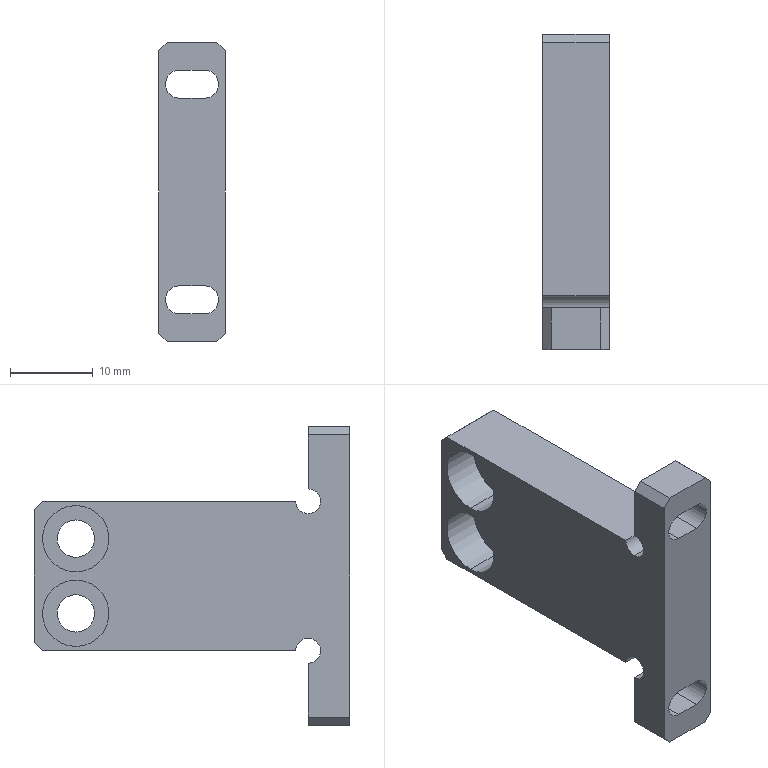Part | SolidWorks | features HoleWzd 2, Chamfer 1, Extrusion 1, ICE 1 | 1 solid | 37 faces | box 8 x 38 x 36 mm | volume 5326 mm3 | plane 22 | cylinder 15 | commonest cylinder face diameters 3.4 x4 4.5 x4 8 x4 3 x3
STEP:
#1=CARTESIAN_POINT('',(4.6,33.,-8.5));
#2=VERTEX_POINT('',#1);
#3=CARTESIAN_POINT('',(4.6,33.,-0.5));
#4=VERTEX_POINT('',#3);
#5=CARTESIAN_POINT('',(4.6,33.,-4.5));
#6=DIRECTION('',(-1.,0.,0.));
#7=DIRECTION('',(0.,0.,1.));
#8=AXIS2_PLACEMENT_3D('',#5,#6,#7);
#9=CIRCLE('',#8,4.);
#10=EDGE_CURVE('',#2,#4,#9,.T.);
#11=ORIENTED_EDGE('',*,*,#10,.F.);
#12=CARTESIAN_POINT('',(0.,33.,-8.5));
#13=VERTEX_POINT('',#12);
#14=CARTESIAN_POINT('',(0.,33.,-8.5));
#15=DIRECTION('',(-1.,0.,0.));
#16=VECTOR('',#15,1000.);
#17=LINE('',#14,#16);
#18=EDGE_CURVE('',#2,#13,#17,.T.);
#19=ORIENTED_EDGE('',*,*,#18,.T.);
#20=CARTESIAN_POINT('',(0.,33.,-0.5));
#21=VERTEX_POINT('',#20);
#22=CARTESIAN_POINT('',(0.,33.,-4.5));
#23=DIRECTION('',(-1.,0.,0.));
#24=DIRECTION('',(0.,0.,1.));
#25=AXIS2_PLACEMENT_3D('',#22,#23,#24);
#26=CIRCLE('',#25,4.);
#27=EDGE_CURVE('',#13,#21,#26,.T.);
#28=ORIENTED_EDGE('',*,*,#27,.T.);
#29=CARTESIAN_POINT('',(0.,33.,-0.5));
#30=DIRECTION('',(-1.,0.,0.));
#31=VECTOR('',#30,1000.);
#32=LINE('',#29,#31);
#33=EDGE_CURVE('',#4,#21,#32,.T.);
#34=ORIENTED_EDGE('',*,*,#33,.F.);
#35=EDGE_LOOP('',(#11,#19,#28,#34));
#36=FACE_OUTER_BOUND('',#35,.T.);
#37=CARTESIAN_POINT('',(0.,33.,-4.5));
#38=DIRECTION('',(-1.,0.,0.));
#39=DIRECTION('',(0.,0.,1.));
#40=AXIS2_PLACEMENT_3D('',#37,#38,#39);
#41=CYLINDRICAL_SURFACE('',#40,4.);
#42=ADVANCED_FACE('',(#36),#41,.F.);
#43=CARTESIAN_POINT('',(8.,33.,-6.75));
#44=VERTEX_POINT('',#43);
#45=CARTESIAN_POINT('',(8.,33.,-2.25));
#46=VERTEX_POINT('',#45);
#47=CARTESIAN_POINT('',(8.,33.,-4.5));
#48=DIRECTION('',(-1.,0.,0.));
#49=DIRECTION('',(0.,0.,1.));
#50=AXIS2_PLACEMENT_3D('',#47,#48,#49);
#51=CIRCLE('',#50,2.25);
#52=EDGE_CURVE('',#44,#46,#51,.T.);
#53=ORIENTED_EDGE('',*,*,#52,.F.);
#54=CARTESIAN_POINT('',(4.6,33.,-6.75));
#55=VERTEX_POINT('',#54);
#56=CARTESIAN_POINT('',(0.,33.,-6.75));
#57=DIRECTION('',(-1.,0.,0.));
#58=VECTOR('',#57,1000.);
#59=LINE('',#56,#58);
#60=EDGE_CURVE('',#44,#55,#59,.T.);
#61=ORIENTED_EDGE('',*,*,#60,.T.);
#62=CARTESIAN_POINT('',(4.6,33.,-2.25));
#63=VERTEX_POINT('',#62);
#64=CARTESIAN_POINT('',(4.6,33.,-4.5));
#65=DIRECTION('',(-1.,0.,0.));
#66=DIRECTION('',(0.,0.,1.));
#67=AXIS2_PLACEMENT_3D('',#64,#65,#66);
#68=CIRCLE('',#67,2.25);
#69=EDGE_CURVE('',#55,#63,#68,.T.);
#70=ORIENTED_EDGE('',*,*,#69,.T.);
#71=CARTESIAN_POINT('',(0.,33.,-2.25));
#72=DIRECTION('',(-1.,0.,0.));
#73=VECTOR('',#72,1000.);
#74=LINE('',#71,#73);
#75=EDGE_CURVE('',#46,#63,#74,.T.);
#76=ORIENTED_EDGE('',*,*,#75,.F.);
#77=EDGE_LOOP('',(#53,#61,#70,#76));
#78=FACE_OUTER_BOUND('',#77,.T.);
#79=CARTESIAN_POINT('',(0.,33.,-4.5));
#80=DIRECTION('',(-1.,0.,0.));
#81=DIRECTION('',(0.,0.,1.));
#82=AXIS2_PLACEMENT_3D('',#79,#80,#81);
#83=CYLINDRICAL_SURFACE('',#82,2.25);
#84=ADVANCED_FACE('',(#78),#83,.F.);
#85=CARTESIAN_POINT('',(4.6,33.,0.5));
#86=VERTEX_POINT('',#85);
#87=CARTESIAN_POINT('',(4.6,33.,8.5));
#88=VERTEX_POINT('',#87);
#89=CARTESIAN_POINT('',(4.6,33.,4.5));
#90=DIRECTION('',(-1.,0.,0.));
#91=DIRECTION('',(0.,0.,1.));
#92=AXIS2_PLACEMENT_3D('',#89,#90,#91);
#93=CIRCLE('',#92,4.);
#94=EDGE_CURVE('',#86,#88,#93,.T.);
#95=ORIENTED_EDGE('',*,*,#94,.F.);
#96=CARTESIAN_POINT('',(0.,33.,0.5));
#97=VERTEX_POINT('',#96);
#98=CARTESIAN_POINT('',(0.,33.,0.5));
#99=DIRECTION('',(-1.,0.,0.));
#100=VECTOR('',#99,1000.);
#101=LINE('',#98,#100);
#102=EDGE_CURVE('',#86,#97,#101,.T.);
#103=ORIENTED_EDGE('',*,*,#102,.T.);
#104=CARTESIAN_POINT('',(0.,33.,8.5));
#105=VERTEX_POINT('',#104);
#106=CARTESIAN_POINT('',(0.,33.,4.5));
#107=DIRECTION('',(-1.,0.,0.));
#108=DIRECTION('',(0.,0.,1.));
#109=AXIS2_PLACEMENT_3D('',#106,#107,#108);
#110=CIRCLE('',#109,4.);
#111=EDGE_CURVE('',#97,#105,#110,.T.);
#112=ORIENTED_EDGE('',*,*,#111,.T.);
#113=CARTESIAN_POINT('',(0.,33.,8.5));
#114=DIRECTION('',(-1.,0.,0.));
#115=VECTOR('',#114,1000.);
#116=LINE('',#113,#115);
#117=EDGE_CURVE('',#88,#105,#116,.T.);
#118=ORIENTED_EDGE('',*,*,#117,.F.);
#119=EDGE_LOOP('',(#95,#103,#112,#118));
#120=FACE_OUTER_BOUND('',#119,.T.);
#121=CARTESIAN_POINT('',(0.,33.,4.5));
#122=DIRECTION('',(-1.,0.,0.));
#123=DIRECTION('',(0.,0.,1.));
#124=AXIS2_PLACEMENT_3D('',#121,#122,#123);
#125=CYLINDRICAL_SURFACE('',#124,4.);
#126=ADVANCED_FACE('',(#120),#125,.F.);
#127=CARTESIAN_POINT('',(8.,33.,2.25));
#128=VERTEX_POINT('',#127);
#129=CARTESIAN_POINT('',(8.,33.,6.75));
#130=VERTEX_POINT('',#129);
#131=CARTESIAN_POINT('',(8.,33.,4.5));
#132=DIRECTION('',(-1.,0.,0.));
#133=DIRECTION('',(0.,0.,1.));
#134=AXIS2_PLACEMENT_3D('',#131,#132,#133);
#135=CIRCLE('',#134,2.25);
#136=EDGE_CURVE('',#128,#130,#135,.T.);
#137=ORIENTED_EDGE('',*,*,#136,.F.);
#138=CARTESIAN_POINT('',(4.6,33.,2.25));
#139=VERTEX_POINT('',#138);
#140=CARTESIAN_POINT('',(0.,33.,2.25));
#141=DIRECTION('',(-1.,0.,0.));
#142=VECTOR('',#141,1000.);
#143=LINE('',#140,#142);
#144=EDGE_CURVE('',#128,#139,#143,.T.);
#145=ORIENTED_EDGE('',*,*,#144,.T.);
#146=CARTESIAN_POINT('',(4.6,33.,6.75));
#147=VERTEX_POINT('',#146);
#148=CARTESIAN_POINT('',(4.6,33.,4.5));
#149=DIRECTION('',(-1.,0.,0.));
#150=DIRECTION('',(0.,0.,1.));
#151=AXIS2_PLACEMENT_3D('',#148,#149,#150);
#152=CIRCLE('',#151,2.25);
#153=EDGE_CURVE('',#139,#147,#152,.T.);
#154=ORIENTED_EDGE('',*,*,#153,.T.);
#155=CARTESIAN_POINT('',(0.,33.,6.75));
#156=DIRECTION('',(-1.,0.,0.));
#157=VECTOR('',#156,1000.);
#158=LINE('',#155,#157);
#159=EDGE_CURVE('',#130,#147,#158,.T.);
#160=ORIENTED_EDGE('',*,*,#159,.F.);
#161=EDGE_LOOP('',(#137,#145,#154,#160));
#162=FACE_OUTER_BOUND('',#161,.T.);
#163=CARTESIAN_POINT('',(0.,33.,4.5));
#164=DIRECTION('',(-1.,0.,0.));
#165=DIRECTION('',(0.,0.,1.));
#166=AXIS2_PLACEMENT_3D('',#163,#164,#165);
#167=CYLINDRICAL_SURFACE('',#166,2.25);
#168=ADVANCED_FACE('',(#162),#167,.F.);
#169=CARTESIAN_POINT('',(0.,5.,7.5));
#170=VERTEX_POINT('',#169);
#171=CARTESIAN_POINT('',(0.,6.5,9.));
#172=VERTEX_POINT('',#171);
#173=CARTESIAN_POINT('',(0.,5.,9.));
#174=DIRECTION('',(1.,0.,0.));
#175=DIRECTION('',(0.,0.,-1.));
#176=AXIS2_PLACEMENT_3D('',#173,#174,#175);
#177=CIRCLE('',#176,1.5);
#178=EDGE_CURVE('',#170,#172,#177,.T.);
#179=ORIENTED_EDGE('',*,*,#178,.F.);
#180=CARTESIAN_POINT('',(8.,5.,7.5));
#181=VERTEX_POINT('',#180);
#182=CARTESIAN_POINT('',(0.,5.,7.5));
#183=DIRECTION('',(1.,0.,0.));
#184=VECTOR('',#183,1000.);
#185=LINE('',#182,#184);
#186=EDGE_CURVE('',#170,#181,#185,.T.);
#187=ORIENTED_EDGE('',*,*,#186,.T.);
#188=CARTESIAN_POINT('',(8.,6.5,9.));
#189=VERTEX_POINT('',#188);
#190=CARTESIAN_POINT('',(8.,5.,9.));
#191=DIRECTION('',(1.,0.,0.));
#192=DIRECTION('',(0.,0.,-1.));
#193=AXIS2_PLACEMENT_3D('',#190,#191,#192);
#194=CIRCLE('',#193,1.5);
#195=EDGE_CURVE('',#181,#189,#194,.T.);
#196=ORIENTED_EDGE('',*,*,#195,.T.);
#197=CARTESIAN_POINT('',(0.,6.5,9.));
#198=DIRECTION('',(1.,0.,0.));
#199=VECTOR('',#198,1000.);
#200=LINE('',#197,#199);
#201=EDGE_CURVE('',#172,#189,#200,.T.);
#202=ORIENTED_EDGE('',*,*,#201,.F.);
#203=EDGE_LOOP('',(#179,#187,#196,#202));
#204=FACE_OUTER_BOUND('',#203,.T.);
#205=CARTESIAN_POINT('',(0.,5.,9.));
#206=DIRECTION('',(1.,0.,0.));
#207=DIRECTION('',(0.,0.,-1.));
#208=AXIS2_PLACEMENT_3D('',#205,#206,#207);
#209=CYLINDRICAL_SURFACE('',#208,1.5);
#210=ADVANCED_FACE('',(#204),#209,.F.);
#211=CARTESIAN_POINT('',(7.,5.,18.));
#212=VERTEX_POINT('',#211);
#213=CARTESIAN_POINT('',(1.,5.,18.));
#214=VERTEX_POINT('',#213);
#215=CARTESIAN_POINT('',(8.,5.,18.));
#216=DIRECTION('',(-1.,0.,0.));
#217=VECTOR('',#216,1000.);
#218=LINE('',#215,#217);
#219=EDGE_CURVE('',#212,#214,#218,.T.);
#220=ORIENTED_EDGE('',*,*,#219,.F.);
#221=CARTESIAN_POINT('',(8.,5.,17.));
#222=VERTEX_POINT('',#221);
#223=CARTESIAN_POINT('',(8.,5.,17.));
#224=DIRECTION('',(0.7071,0.,-0.7071));
#225=VECTOR('',#224,1000.);
#226=LINE('',#223,#225);
#227=EDGE_CURVE('',#212,#222,#226,.T.);
#228=ORIENTED_EDGE('',*,*,#227,.T.);
#229=CARTESIAN_POINT('',(8.,5.,10.5));
#230=VERTEX_POINT('',#229);
#231=CARTESIAN_POINT('',(8.,5.,9.));
#232=DIRECTION('',(0.,0.,1.));
#233=VECTOR('',#232,1000.);
#234=LINE('',#231,#233);
#235=EDGE_CURVE('',#230,#222,#234,.T.);
#236=ORIENTED_EDGE('',*,*,#235,.F.);
#237=CARTESIAN_POINT('',(0.,5.,10.5));
#238=VERTEX_POINT('',#237);
#239=CARTESIAN_POINT('',(0.,5.,10.5));
#240=DIRECTION('',(-1.,0.,0.));
#241=VECTOR('',#240,1000.);
#242=LINE('',#239,#241);
#243=EDGE_CURVE('',#230,#238,#242,.T.);
#244=ORIENTED_EDGE('',*,*,#243,.T.);
#245=CARTESIAN_POINT('',(0.,5.,17.));
#246=VERTEX_POINT('',#245);
#247=CARTESIAN_POINT('',(0.,5.,9.));
#248=DIRECTION('',(0.,0.,1.));
#249=VECTOR('',#248,1000.);
#250=LINE('',#247,#249);
#251=EDGE_CURVE('',#238,#246,#250,.T.);
#252=ORIENTED_EDGE('',*,*,#251,.T.);
#253=CARTESIAN_POINT('',(1.,5.,18.));
#254=DIRECTION('',(0.7071,0.,0.7071));
#255=VECTOR('',#254,1000.);
#256=LINE('',#253,#255);
#257=EDGE_CURVE('',#246,#214,#256,.T.);
#258=ORIENTED_EDGE('',*,*,#257,.T.);
#259=EDGE_LOOP('',(#220,#228,#236,#244,#252,#258));
#260=FACE_OUTER_BOUND('',#259,.T.);
#261=CARTESIAN_POINT('',(2.5,5.,11.3));
#262=VERTEX_POINT('',#261);
#263=CARTESIAN_POINT('',(2.5,5.,14.7));
#264=VERTEX_POINT('',#263);
#265=CARTESIAN_POINT('',(2.5,5.,13.));
#266=DIRECTION('',(0.,1.,0.));
#267=DIRECTION('',(0.,0.,1.));
#268=AXIS2_PLACEMENT_3D('',#265,#266,#267);
#269=CIRCLE('',#268,1.7);
#270=EDGE_CURVE('',#262,#264,#269,.T.);
#271=ORIENTED_EDGE('',*,*,#270,.F.);
#272=CARTESIAN_POINT('',(5.5,5.,11.3));
#273=VERTEX_POINT('',#272);
#274=CARTESIAN_POINT('',(2.5,5.,11.3));
#275=DIRECTION('',(1.,0.,0.));
#276=VECTOR('',#275,1000.);
#277=LINE('',#274,#276);
#278=EDGE_CURVE('',#262,#273,#277,.T.);
#279=ORIENTED_EDGE('',*,*,#278,.T.);
#280=CARTESIAN_POINT('',(5.5,5.,14.7));
#281=VERTEX_POINT('',#280);
#282=CARTESIAN_POINT('',(5.5,5.,13.));
#283=DIRECTION('',(0.,1.,0.));
#284=DIRECTION('',(0.,0.,1.));
#285=AXIS2_PLACEMENT_3D('',#282,#283,#284);
#286=CIRCLE('',#285,1.7);
#287=EDGE_CURVE('',#281,#273,#286,.T.);
#288=ORIENTED_EDGE('',*,*,#287,.F.);
#289=CARTESIAN_POINT('',(2.5,5.,14.7));
#290=DIRECTION('',(1.,0.,0.));
#291=VECTOR('',#290,1000.);
#292=LINE('',#289,#291);
#293=EDGE_CURVE('',#264,#281,#292,.T.);
#294=ORIENTED_EDGE('',*,*,#293,.F.);
#295=EDGE_LOOP('',(#271,#279,#288,#294));
#296=FACE_BOUND('',#295,.T.);
#297=CARTESIAN_POINT('',(8.,5.,9.));
#298=DIRECTION('',(0.,-1.,0.));
#299=DIRECTION('',(0.,0.,-1.));
#300=AXIS2_PLACEMENT_3D('',#297,#298,#299);
#301=PLANE('',#300);
#302=ADVANCED_FACE('',(#260,#296),#301,.F.);
#303=CARTESIAN_POINT('',(0.,6.5,-9.));
#304=VERTEX_POINT('',#303);
#305=CARTESIAN_POINT('',(0.,37.,-9.));
#306=VERTEX_POINT('',#305);
#307=CARTESIAN_POINT('',(0.,38.,-9.));
#308=DIRECTION('',(0.,1.,0.));
#309=VECTOR('',#308,1000.);
#310=LINE('',#307,#309);
#311=EDGE_CURVE('',#304,#306,#310,.T.);
#312=ORIENTED_EDGE('',*,*,#311,.T.);
#313=CARTESIAN_POINT('',(8.,37.,-9.));
#314=VERTEX_POINT('',#313);
#315=CARTESIAN_POINT('',(8.,37.,-9.));
#316=DIRECTION('',(1.,0.,0.));
#317=VECTOR('',#316,1000.);
#318=LINE('',#315,#317);
#319=EDGE_CURVE('',#306,#314,#318,.T.);
#320=ORIENTED_EDGE('',*,*,#319,.T.);
#321=CARTESIAN_POINT('',(8.,6.5,-9.));
#322=VERTEX_POINT('',#321);
#323=CARTESIAN_POINT('',(8.,38.,-9.));
#324=DIRECTION('',(0.,1.,0.));
#325=VECTOR('',#324,1000.);
#326=LINE('',#323,#325);
#327=EDGE_CURVE('',#322,#314,#326,.T.);
#328=ORIENTED_EDGE('',*,*,#327,.F.);
#329=CARTESIAN_POINT('',(0.,6.5,-9.));
#330=DIRECTION('',(-1.,0.,0.));
#331=VECTOR('',#330,1000.);
#332=LINE('',#329,#331);
#333=EDGE_CURVE('',#322,#304,#332,.T.);
#334=ORIENTED_EDGE('',*,*,#333,.T.);
#335=EDGE_LOOP('',(#312,#320,#328,#334));
#336=FACE_OUTER_BOUND('',#335,.T.);
#337=CARTESIAN_POINT('',(8.,38.,-9.));
#338=DIRECTION('',(0.,0.,1.));
#339=DIRECTION('',(0.,-1.,0.));
#340=AXIS2_PLACEMENT_3D('',#337,#338,#339);
#341=PLANE('',#340);
#342=ADVANCED_FACE('',(#336),#341,.F.);
#343=CARTESIAN_POINT('',(0.,38.,-8.));
#344=VERTEX_POINT('',#343);
#345=CARTESIAN_POINT('',(0.,38.,8.));
#346=VERTEX_POINT('',#345);
#347=CARTESIAN_POINT('',(0.,38.,9.));
#348=DIRECTION('',(0.,0.,1.));
#349=VECTOR('',#348,1000.);
#350=LINE('',#347,#349);
#351=EDGE_CURVE('',#344,#346,#350,.T.);
#352=ORIENTED_EDGE('',*,*,#351,.T.);
#353=CARTESIAN_POINT('',(8.,38.,8.));
#354=VERTEX_POINT('',#353);
#355=CARTESIAN_POINT('',(8.,38.,8.));
#356=DIRECTION('',(1.,0.,0.));
#357=VECTOR('',#356,1000.);
#358=LINE('',#355,#357);
#359=EDGE_CURVE('',#346,#354,#358,.T.);
#360=ORIENTED_EDGE('',*,*,#359,.T.);
#361=CARTESIAN_POINT('',(8.,38.,-8.));
#362=VERTEX_POINT('',#361);
#363=CARTESIAN_POINT('',(8.,38.,9.));
#364=DIRECTION('',(0.,0.,1.));
#365=VECTOR('',#364,1000.);
#366=LINE('',#363,#365);
#367=EDGE_CURVE('',#362,#354,#366,.T.);
#368=ORIENTED_EDGE('',*,*,#367,.F.);
#369=CARTESIAN_POINT('',(8.,38.,-8.));
#370=DIRECTION('',(-1.,0.,0.));
#371=VECTOR('',#370,1000.);
#372=LINE('',#369,#371);
#373=EDGE_CURVE('',#362,#344,#372,.T.);
#374=ORIENTED_EDGE('',*,*,#373,.T.);
#375=EDGE_LOOP('',(#352,#360,#368,#374));
#376=FACE_OUTER_BOUND('',#375,.T.);
#377=CARTESIAN_POINT('',(8.,38.,9.));
#378=DIRECTION('',(0.,-1.,0.));
#379=DIRECTION('',(0.,0.,-1.));
#380=AXIS2_PLACEMENT_3D('',#377,#378,#379);
#381=PLANE('',#380);
#382=ADVANCED_FACE('',(#376),#381,.F.);
#383=CARTESIAN_POINT('',(8.,37.,9.));
#384=VERTEX_POINT('',#383);
#385=CARTESIAN_POINT('',(8.,38.,9.));
#386=DIRECTION('',(0.,-1.,0.));
#387=VECTOR('',#386,1000.);
#388=LINE('',#385,#387);
#389=EDGE_CURVE('',#384,#189,#388,.T.);
#390=ORIENTED_EDGE('',*,*,#389,.F.);
#391=CARTESIAN_POINT('',(0.,37.,9.));
#392=VERTEX_POINT('',#391);
#393=CARTESIAN_POINT('',(8.,37.,9.));
#394=DIRECTION('',(-1.,0.,0.));
#395=VECTOR('',#394,1000.);
#396=LINE('',#393,#395);
#397=EDGE_CURVE('',#384,#392,#396,.T.);
#398=ORIENTED_EDGE('',*,*,#397,.T.);
#399=CARTESIAN_POINT('',(0.,38.,9.));
#400=DIRECTION('',(0.,-1.,0.));
#401=VECTOR('',#400,1000.);
#402=LINE('',#399,#401);
#403=EDGE_CURVE('',#392,#172,#402,.T.);
#404=ORIENTED_EDGE('',*,*,#403,.T.);
#405=ORIENTED_EDGE('',*,*,#201,.T.);
#406=EDGE_LOOP('',(#390,#398,#404,#405));
#407=FACE_OUTER_BOUND('',#406,.T.);
#408=CARTESIAN_POINT('',(8.,38.,9.));
#409=DIRECTION('',(0.,0.,-1.));
#410=DIRECTION('',(0.,1.,0.));
#411=AXIS2_PLACEMENT_3D('',#408,#409,#410);
#412=PLANE('',#411);
#413=ADVANCED_FACE('',(#407),#412,.F.);
#414=CARTESIAN_POINT('',(7.,0.,18.));
#415=VERTEX_POINT('',#414);
#416=CARTESIAN_POINT('',(1.,0.,18.));
#417=VERTEX_POINT('',#416);
#418=CARTESIAN_POINT('',(8.,0.,18.));
#419=DIRECTION('',(-1.,0.,0.));
#420=VECTOR('',#419,1000.);
#421=LINE('',#418,#420);
#422=EDGE_CURVE('',#415,#417,#421,.T.);
#423=ORIENTED_EDGE('',*,*,#422,.F.);
#424=CARTESIAN_POINT('',(7.,5.,18.));
#425=DIRECTION('',(0.,1.,0.));
#426=VECTOR('',#425,1000.);
#427=LINE('',#424,#426);
#428=EDGE_CURVE('',#415,#212,#427,.T.);
#429=ORIENTED_EDGE('',*,*,#428,.T.);
#430=ORIENTED_EDGE('',*,*,#219,.T.);
#431=CARTESIAN_POINT('',(1.,5.,18.));
#432=DIRECTION('',(0.,-1.,0.));
#433=VECTOR('',#432,1000.);
#434=LINE('',#431,#433);
#435=EDGE_CURVE('',#214,#417,#434,.T.);
#436=ORIENTED_EDGE('',*,*,#435,.T.);
#437=EDGE_LOOP('',(#423,#429,#430,#436));
#438=FACE_OUTER_BOUND('',#437,.T.);
#439=CARTESIAN_POINT('',(8.,5.,18.));
#440=DIRECTION('',(0.,0.,-1.));
#441=DIRECTION('',(-1.,0.,0.));
#442=AXIS2_PLACEMENT_3D('',#439,#440,#441);
#443=PLANE('',#442);
#444=ADVANCED_FACE('',(#438),#443,.F.);
#445=CARTESIAN_POINT('',(2.5,0.,-11.3));
#446=VERTEX_POINT('',#445);
#447=CARTESIAN_POINT('',(5.5,0.,-11.3));
#448=VERTEX_POINT('',#447);
#449=CARTESIAN_POINT('',(2.5,0.,-11.3));
#450=DIRECTION('',(1.,0.,0.));
#451=VECTOR('',#450,1000.);
#452=LINE('',#449,#451);
#453=EDGE_CURVE('',#446,#448,#452,.T.);
#454=ORIENTED_EDGE('',*,*,#453,.T.);
#455=CARTESIAN_POINT('',(5.5,0.,-14.7));
#456=VERTEX_POINT('',#455);
#457=CARTESIAN_POINT('',(5.5,0.,-13.));
#458=DIRECTION('',(0.,1.,0.));
#459=DIRECTION('',(0.,0.,1.));
#460=AXIS2_PLACEMENT_3D('',#457,#458,#459);
#461=CIRCLE('',#460,1.7);
#462=EDGE_CURVE('',#448,#456,#461,.T.);
#463=ORIENTED_EDGE('',*,*,#462,.T.);
#464=CARTESIAN_POINT('',(2.5,0.,-14.7));
#465=VERTEX_POINT('',#464);
#466=CARTESIAN_POINT('',(2.5,0.,-14.7));
#467=DIRECTION('',(1.,0.,0.));
#468=VECTOR('',#467,1000.);
#469=LINE('',#466,#468);
#470=EDGE_CURVE('',#465,#456,#469,.T.);
#471=ORIENTED_EDGE('',*,*,#470,.F.);
#472=CARTESIAN_POINT('',(2.5,0.,-13.));
#473=DIRECTION('',(0.,1.,0.));
#474=DIRECTION('',(0.,0.,1.));
#475=AXIS2_PLACEMENT_3D('',#472,#473,#474);
#476=CIRCLE('',#475,1.7);
#477=EDGE_CURVE('',#465,#446,#476,.T.);
#478=ORIENTED_EDGE('',*,*,#477,.T.);
#479=EDGE_LOOP('',(#454,#463,#471,#478));
#480=FACE_BOUND('',#479,.T.);
#481=CARTESIAN_POINT('',(2.5,0.,11.3));
#482=VERTEX_POINT('',#481);
#483=CARTESIAN_POINT('',(2.5,0.,14.7));
#484=VERTEX_POINT('',#483);
#485=CARTESIAN_POINT('',(2.5,0.,13.));
#486=DIRECTION('',(0.,1.,0.));
#487=DIRECTION('',(0.,0.,1.));
#488=AXIS2_PLACEMENT_3D('',#485,#486,#487);
#489=CIRCLE('',#488,1.7);
#490=EDGE_CURVE('',#482,#484,#489,.T.);
#491=ORIENTED_EDGE('',*,*,#490,.T.);
#492=CARTESIAN_POINT('',(5.5,0.,14.7));
#493=VERTEX_POINT('',#492);
#494=CARTESIAN_POINT('',(2.5,0.,14.7));
#495=DIRECTION('',(1.,0.,0.));
#496=VECTOR('',#495,1000.);
#497=LINE('',#494,#496);
#498=EDGE_CURVE('',#484,#493,#497,.T.);
#499=ORIENTED_EDGE('',*,*,#498,.T.);
#500=CARTESIAN_POINT('',(5.5,0.,11.3));
#501=VERTEX_POINT('',#500);
#502=CARTESIAN_POINT('',(5.5,0.,13.));
#503=DIRECTION('',(0.,1.,0.));
#504=DIRECTION('',(0.,0.,1.));
#505=AXIS2_PLACEMENT_3D('',#502,#503,#504);
#506=CIRCLE('',#505,1.7);
#507=EDGE_CURVE('',#493,#501,#506,.T.);
#508=ORIENTED_EDGE('',*,*,#507,.T.);
#509=CARTESIAN_POINT('',(2.5,0.,11.3));
#510=DIRECTION('',(1.,0.,0.));
#511=VECTOR('',#510,1000.);
#512=LINE('',#509,#511);
#513=EDGE_CURVE('',#482,#501,#512,.T.);
#514=ORIENTED_EDGE('',*,*,#513,.F.);
#515=EDGE_LOOP('',(#491,#499,#508,#514));
#516=FACE_BOUND('',#515,.T.);
#517=CARTESIAN_POINT('',(7.,0.,-18.));
#518=VERTEX_POINT('',#517);
#519=CARTESIAN_POINT('',(1.,0.,-18.));
#520=VERTEX_POINT('',#519);
#521=CARTESIAN_POINT('',(8.,0.,-18.));
#522=DIRECTION('',(-1.,0.,0.));
#523=VECTOR('',#522,1000.);
#524=LINE('',#521,#523);
#525=EDGE_CURVE('',#518,#520,#524,.T.);
#526=ORIENTED_EDGE('',*,*,#525,.F.);
#527=CARTESIAN_POINT('',(8.,0.,-17.));
#528=VERTEX_POINT('',#527);
#529=CARTESIAN_POINT('',(8.,0.,-17.));
#530=DIRECTION('',(0.7071,0.,0.7071));
#531=VECTOR('',#530,1000.);
#532=LINE('',#529,#531);
#533=EDGE_CURVE('',#518,#528,#532,.T.);
#534=ORIENTED_EDGE('',*,*,#533,.T.);
#535=CARTESIAN_POINT('',(8.,0.,17.));
#536=VERTEX_POINT('',#535);
#537=CARTESIAN_POINT('',(8.,0.,-18.));
#538=DIRECTION('',(0.,0.,-1.));
#539=VECTOR('',#538,1000.);
#540=LINE('',#537,#539);
#541=EDGE_CURVE('',#536,#528,#540,.T.);
#542=ORIENTED_EDGE('',*,*,#541,.F.);
#543=CARTESIAN_POINT('',(8.,0.,17.));
#544=DIRECTION('',(-0.7071,0.,0.7071));
#545=VECTOR('',#544,1000.);
#546=LINE('',#543,#545);
#547=EDGE_CURVE('',#536,#415,#546,.T.);
#548=ORIENTED_EDGE('',*,*,#547,.T.);
#549=ORIENTED_EDGE('',*,*,#422,.T.);
#550=CARTESIAN_POINT('',(0.,0.,17.));
#551=VERTEX_POINT('',#550);
#552=CARTESIAN_POINT('',(1.,0.,18.));
#553=DIRECTION('',(-0.7071,0.,-0.7071));
#554=VECTOR('',#553,1000.);
#555=LINE('',#552,#554);
#556=EDGE_CURVE('',#417,#551,#555,.T.);
#557=ORIENTED_EDGE('',*,*,#556,.T.);
#558=CARTESIAN_POINT('',(0.,0.,-17.));
#559=VERTEX_POINT('',#558);
#560=CARTESIAN_POINT('',(0.,0.,-18.));
#561=DIRECTION('',(0.,0.,-1.));
#562=VECTOR('',#561,1000.);
#563=LINE('',#560,#562);
#564=EDGE_CURVE('',#551,#559,#563,.T.);
#565=ORIENTED_EDGE('',*,*,#564,.T.);
#566=CARTESIAN_POINT('',(1.,0.,-18.));
#567=DIRECTION('',(0.7071,0.,-0.7071));
#568=VECTOR('',#567,1000.);
#569=LINE('',#566,#568);
#570=EDGE_CURVE('',#559,#520,#569,.T.);
#571=ORIENTED_EDGE('',*,*,#570,.T.);
#572=EDGE_LOOP('',(#526,#534,#542,#548,#549,#557,#565,#571));
#573=FACE_OUTER_BOUND('',#572,.T.);
#574=CARTESIAN_POINT('',(8.,0.,-18.));
#575=DIRECTION('',(0.,1.,0.));
#576=DIRECTION('',(0.,0.,1.));
#577=AXIS2_PLACEMENT_3D('',#574,#575,#576);
#578=PLANE('',#577);
#579=ADVANCED_FACE('',(#480,#516,#573),#578,.F.);
#580=CARTESIAN_POINT('',(7.,5.,-18.));
#581=VERTEX_POINT('',#580);
#582=CARTESIAN_POINT('',(1.,5.,-18.));
#583=VERTEX_POINT('',#582);
#584=CARTESIAN_POINT('',(8.,5.,-18.));
#585=DIRECTION('',(-1.,0.,0.));
#586=VECTOR('',#585,1000.);
#587=LINE('',#584,#586);
#588=EDGE_CURVE('',#581,#583,#587,.T.);
#589=ORIENTED_EDGE('',*,*,#588,.F.);
#590=CARTESIAN_POINT('',(7.,0.,-18.));
#591=DIRECTION('',(0.,-1.,0.));
#592=VECTOR('',#591,1000.);
#593=LINE('',#590,#592);
#594=EDGE_CURVE('',#581,#518,#593,.T.);
#595=ORIENTED_EDGE('',*,*,#594,.T.);
#596=ORIENTED_EDGE('',*,*,#525,.T.);
#597=CARTESIAN_POINT('',(1.,5.,-18.));
#598=DIRECTION('',(0.,1.,0.));
#599=VECTOR('',#598,1000.);
#600=LINE('',#597,#599);
#601=EDGE_CURVE('',#520,#583,#600,.T.);
#602=ORIENTED_EDGE('',*,*,#601,.T.);
#603=EDGE_LOOP('',(#589,#595,#596,#602));
#604=FACE_OUTER_BOUND('',#603,.T.);
#605=CARTESIAN_POINT('',(8.,5.,-18.));
#606=DIRECTION('',(0.,0.,1.));
#607=DIRECTION('',(1.,0.,0.));
#608=AXIS2_PLACEMENT_3D('',#605,#606,#607);
#609=PLANE('',#608);
#610=ADVANCED_FACE('',(#604),#609,.F.);
#611=CARTESIAN_POINT('',(2.5,5.,-14.7));
#612=VERTEX_POINT('',#611);
#613=CARTESIAN_POINT('',(2.5,5.,-11.3));
#614=VERTEX_POINT('',#613);
#615=CARTESIAN_POINT('',(2.5,5.,-13.));
#616=DIRECTION('',(0.,1.,0.));
#617=DIRECTION('',(0.,0.,1.));
#618=AXIS2_PLACEMENT_3D('',#615,#616,#617);
#619=CIRCLE('',#618,1.7);
#620=EDGE_CURVE('',#612,#614,#619,.T.);
#621=ORIENTED_EDGE('',*,*,#620,.F.);
#622=CARTESIAN_POINT('',(5.5,5.,-14.7));
#623=VERTEX_POINT('',#622);
#624=CARTESIAN_POINT('',(2.5,5.,-14.7));
#625=DIRECTION('',(1.,0.,0.));
#626=VECTOR('',#625,1000.);
#627=LINE('',#624,#626);
#628=EDGE_CURVE('',#612,#623,#627,.T.);
#629=ORIENTED_EDGE('',*,*,#628,.T.);
#630=CARTESIAN_POINT('',(5.5,5.,-11.3));
#631=VERTEX_POINT('',#630);
#632=CARTESIAN_POINT('',(5.5,5.,-13.));
#633=DIRECTION('',(0.,1.,0.));
#634=DIRECTION('',(0.,0.,1.));
#635=AXIS2_PLACEMENT_3D('',#632,#633,#634);
#636=CIRCLE('',#635,1.7);
#637=EDGE_CURVE('',#631,#623,#636,.T.);
#638=ORIENTED_EDGE('',*,*,#637,.F.);
#639=CARTESIAN_POINT('',(2.5,5.,-11.3));
#640=DIRECTION('',(1.,0.,0.));
#641=VECTOR('',#640,1000.);
#642=LINE('',#639,#641);
#643=EDGE_CURVE('',#614,#631,#642,.T.);
#644=ORIENTED_EDGE('',*,*,#643,.F.);
#645=EDGE_LOOP('',(#621,#629,#638,#644));
#646=FACE_BOUND('',#645,.T.);
#647=CARTESIAN_POINT('',(8.,5.,-17.));
#648=VERTEX_POINT('',#647);
#649=CARTESIAN_POINT('',(8.,5.,-10.5));
#650=VERTEX_POINT('',#649);
#651=CARTESIAN_POINT('',(8.,5.,-9.));
#652=DIRECTION('',(0.,0.,1.));
#653=VECTOR('',#652,1000.);
#654=LINE('',#651,#653);
#655=EDGE_CURVE('',#648,#650,#654,.T.);
#656=ORIENTED_EDGE('',*,*,#655,.F.);
#657=CARTESIAN_POINT('',(8.,5.,-17.));
#658=DIRECTION('',(-0.7071,0.,-0.7071));
#659=VECTOR('',#658,1000.);
#660=LINE('',#657,#659);
#661=EDGE_CURVE('',#648,#581,#660,.T.);
#662=ORIENTED_EDGE('',*,*,#661,.T.);
#663=ORIENTED_EDGE('',*,*,#588,.T.);
#664=CARTESIAN_POINT('',(0.,5.,-17.));
#665=VERTEX_POINT('',#664);
#666=CARTESIAN_POINT('',(1.,5.,-18.));
#667=DIRECTION('',(-0.7071,0.,0.7071));
#668=VECTOR('',#667,1000.);
#669=LINE('',#666,#668);
#670=EDGE_CURVE('',#583,#665,#669,.T.);
#671=ORIENTED_EDGE('',*,*,#670,.T.);
#672=CARTESIAN_POINT('',(0.,5.,-10.5));
#673=VERTEX_POINT('',#672);
#674=CARTESIAN_POINT('',(0.,5.,-9.));
#675=DIRECTION('',(0.,0.,1.));
#676=VECTOR('',#675,1000.);
#677=LINE('',#674,#676);
#678=EDGE_CURVE('',#665,#673,#677,.T.);
#679=ORIENTED_EDGE('',*,*,#678,.T.);
#680=CARTESIAN_POINT('',(0.,5.,-10.5));
#681=DIRECTION('',(1.,0.,0.));
#682=VECTOR('',#681,1000.);
#683=LINE('',#680,#682);
#684=EDGE_CURVE('',#673,#650,#683,.T.);
#685=ORIENTED_EDGE('',*,*,#684,.T.);
#686=EDGE_LOOP('',(#656,#662,#663,#671,#679,#685));
#687=FACE_OUTER_BOUND('',#686,.T.);
#688=CARTESIAN_POINT('',(8.,5.,-9.));
#689=DIRECTION('',(0.,-1.,0.));
#690=DIRECTION('',(0.,0.,-1.));
#691=AXIS2_PLACEMENT_3D('',#688,#689,#690);
#692=PLANE('',#691);
#693=ADVANCED_FACE('',(#646,#687),#692,.F.);
#694=CARTESIAN_POINT('',(8.,33.,-4.5));
#695=DIRECTION('',(-1.,0.,0.));
#696=DIRECTION('',(0.,0.,1.));
#697=AXIS2_PLACEMENT_3D('',#694,#695,#696);
#698=CIRCLE('',#697,2.25);
#699=EDGE_CURVE('',#46,#44,#698,.T.);
#700=ORIENTED_EDGE('',*,*,#699,.T.);
#701=ORIENTED_EDGE('',*,*,#52,.T.);
#702=EDGE_LOOP('',(#700,#701));
#703=FACE_BOUND('',#702,.T.);
#704=CARTESIAN_POINT('',(8.,33.,4.5));
#705=DIRECTION('',(-1.,0.,0.));
#706=DIRECTION('',(0.,0.,1.));
#707=AXIS2_PLACEMENT_3D('',#704,#705,#706);
#708=CIRCLE('',#707,2.25);
#709=EDGE_CURVE('',#130,#128,#708,.T.);
#710=ORIENTED_EDGE('',*,*,#709,.T.);
#711=ORIENTED_EDGE('',*,*,#136,.T.);
#712=EDGE_LOOP('',(#710,#711));
#713=FACE_BOUND('',#712,.T.);
#714=ORIENTED_EDGE('',*,*,#541,.T.);
#715=CARTESIAN_POINT('',(8.,5.,-17.));
#716=DIRECTION('',(0.,1.,0.));
#717=VECTOR('',#716,1000.);
#718=LINE('',#715,#717);
#719=EDGE_CURVE('',#528,#648,#718,.T.);
#720=ORIENTED_EDGE('',*,*,#719,.T.);
#721=ORIENTED_EDGE('',*,*,#655,.T.);
#722=CARTESIAN_POINT('',(8.,5.,-9.));
#723=DIRECTION('',(1.,0.,0.));
#724=DIRECTION('',(0.,0.,1.));
#725=AXIS2_PLACEMENT_3D('',#722,#723,#724);
#726=CIRCLE('',#725,1.5);
#727=EDGE_CURVE('',#322,#650,#726,.T.);
#728=ORIENTED_EDGE('',*,*,#727,.F.);
#729=ORIENTED_EDGE('',*,*,#327,.T.);
#730=CARTESIAN_POINT('',(8.,23.,-23.));
#731=DIRECTION('',(0.,0.7071,0.7071));
#732=VECTOR('',#731,1000.);
#733=LINE('',#730,#732);
#734=EDGE_CURVE('',#314,#362,#733,.T.);
#735=ORIENTED_EDGE('',*,*,#734,.T.);
#736=ORIENTED_EDGE('',*,*,#367,.T.);
#737=CARTESIAN_POINT('',(8.,23.,23.));
#738=DIRECTION('',(0.,-0.7071,0.7071));
#739=VECTOR('',#738,1000.);
#740=LINE('',#737,#739);
#741=EDGE_CURVE('',#354,#384,#740,.T.);
#742=ORIENTED_EDGE('',*,*,#741,.T.);
#743=ORIENTED_EDGE('',*,*,#389,.T.);
#744=ORIENTED_EDGE('',*,*,#195,.F.);
#745=CARTESIAN_POINT('',(8.,5.,9.));
#746=DIRECTION('',(1.,0.,0.));
#747=DIRECTION('',(0.,0.,-1.));
#748=AXIS2_PLACEMENT_3D('',#745,#746,#747);
#749=CIRCLE('',#748,1.5);
#750=EDGE_CURVE('',#230,#181,#749,.T.);
#751=ORIENTED_EDGE('',*,*,#750,.F.);
#752=ORIENTED_EDGE('',*,*,#235,.T.);
#753=CARTESIAN_POINT('',(8.,0.,17.));
#754=DIRECTION('',(0.,-1.,0.));
#755=VECTOR('',#754,1000.);
#756=LINE('',#753,#755);
#757=EDGE_CURVE('',#222,#536,#756,.T.);
#758=ORIENTED_EDGE('',*,*,#757,.T.);
#759=EDGE_LOOP('',(#714,#720,#721,#728,#729,#735,#736,#742,#743,#744,#751,#752,#758));
#760=FACE_OUTER_BOUND('',#759,.T.);
#761=CARTESIAN_POINT('',(8.,0.,0.));
#762=DIRECTION('',(1.,0.,0.));
#763=DIRECTION('',(0.,0.,-1.));
#764=AXIS2_PLACEMENT_3D('',#761,#762,#763);
#765=PLANE('',#764);
#766=ADVANCED_FACE('',(#703,#713,#760),#765,.T.);
#767=CARTESIAN_POINT('',(0.,33.,-4.5));
#768=DIRECTION('',(-1.,0.,0.));
#769=DIRECTION('',(0.,0.,1.));
#770=AXIS2_PLACEMENT_3D('',#767,#768,#769);
#771=CIRCLE('',#770,4.);
#772=EDGE_CURVE('',#21,#13,#771,.T.);
#773=ORIENTED_EDGE('',*,*,#772,.F.);
#774=ORIENTED_EDGE('',*,*,#27,.F.);
#775=EDGE_LOOP('',(#773,#774));
#776=FACE_BOUND('',#775,.T.);
#777=CARTESIAN_POINT('',(0.,33.,4.5));
#778=DIRECTION('',(-1.,0.,0.));
#779=DIRECTION('',(0.,0.,1.));
#780=AXIS2_PLACEMENT_3D('',#777,#778,#779);
#781=CIRCLE('',#780,4.);
#782=EDGE_CURVE('',#105,#97,#781,.T.);
#783=ORIENTED_EDGE('',*,*,#782,.F.);
#784=ORIENTED_EDGE('',*,*,#111,.F.);
#785=EDGE_LOOP('',(#783,#784));
#786=FACE_BOUND('',#785,.T.);
#787=ORIENTED_EDGE('',*,*,#678,.F.);
#788=CARTESIAN_POINT('',(0.,0.,-17.));
#789=DIRECTION('',(0.,-1.,0.));
#790=VECTOR('',#789,1000.);
#791=LINE('',#788,#790);
#792=EDGE_CURVE('',#665,#559,#791,.T.);
#793=ORIENTED_EDGE('',*,*,#792,.T.);
#794=ORIENTED_EDGE('',*,*,#564,.F.);
#795=CARTESIAN_POINT('',(0.,0.,17.));
#796=DIRECTION('',(0.,1.,0.));
#797=VECTOR('',#796,1000.);
#798=LINE('',#795,#797);
#799=EDGE_CURVE('',#551,#246,#798,.T.);
#800=ORIENTED_EDGE('',*,*,#799,.T.);
#801=ORIENTED_EDGE('',*,*,#251,.F.);
#802=CARTESIAN_POINT('',(0.,5.,9.));
#803=DIRECTION('',(1.,0.,0.));
#804=DIRECTION('',(0.,0.,-1.));
#805=AXIS2_PLACEMENT_3D('',#802,#803,#804);
#806=CIRCLE('',#805,1.5);
#807=EDGE_CURVE('',#238,#170,#806,.T.);
#808=ORIENTED_EDGE('',*,*,#807,.T.);
#809=ORIENTED_EDGE('',*,*,#178,.T.);
#810=ORIENTED_EDGE('',*,*,#403,.F.);
#811=CARTESIAN_POINT('',(0.,37.,9.));
#812=DIRECTION('',(0.,0.7071,-0.7071));
#813=VECTOR('',#812,1000.);
#814=LINE('',#811,#813);
#815=EDGE_CURVE('',#392,#346,#814,.T.);
#816=ORIENTED_EDGE('',*,*,#815,.T.);
#817=ORIENTED_EDGE('',*,*,#351,.F.);
#818=CARTESIAN_POINT('',(0.,38.,-8.));
#819=DIRECTION('',(0.,-0.7071,-0.7071));
#820=VECTOR('',#819,1000.);
#821=LINE('',#818,#820);
#822=EDGE_CURVE('',#344,#306,#821,.T.);
#823=ORIENTED_EDGE('',*,*,#822,.T.);
#824=ORIENTED_EDGE('',*,*,#311,.F.);
#825=CARTESIAN_POINT('',(0.,5.,-9.));
#826=DIRECTION('',(1.,0.,0.));
#827=DIRECTION('',(0.,0.,-1.));
#828=AXIS2_PLACEMENT_3D('',#825,#826,#827);
#829=CIRCLE('',#828,1.5);
#830=EDGE_CURVE('',#304,#673,#829,.T.);
#831=ORIENTED_EDGE('',*,*,#830,.T.);
#832=EDGE_LOOP('',(#787,#793,#794,#800,#801,#808,#809,#810,#816,#817,#823,#824,#831));
#833=FACE_OUTER_BOUND('',#832,.T.);
#834=CARTESIAN_POINT('',(0.,0.,0.));
#835=DIRECTION('',(1.,0.,0.));
#836=DIRECTION('',(0.,0.,-1.));
#837=AXIS2_PLACEMENT_3D('',#834,#835,#836);
#838=PLANE('',#837);
#839=ADVANCED_FACE('',(#776,#786,#833),#838,.F.);
#840=ORIENTED_EDGE('',*,*,#727,.T.);
#841=ORIENTED_EDGE('',*,*,#684,.F.);
#842=ORIENTED_EDGE('',*,*,#830,.F.);
#843=ORIENTED_EDGE('',*,*,#333,.F.);
#844=EDGE_LOOP('',(#840,#841,#842,#843));
#845=FACE_OUTER_BOUND('',#844,.T.);
#846=CARTESIAN_POINT('',(0.,5.,-9.));
#847=DIRECTION('',(1.,0.,0.));
#848=DIRECTION('',(0.,0.,-1.));
#849=AXIS2_PLACEMENT_3D('',#846,#847,#848);
#850=CYLINDRICAL_SURFACE('',#849,1.5);
#851=ADVANCED_FACE('',(#845),#850,.F.);
#852=ORIENTED_EDGE('',*,*,#186,.F.);
#853=ORIENTED_EDGE('',*,*,#807,.F.);
#854=ORIENTED_EDGE('',*,*,#243,.F.);
#855=ORIENTED_EDGE('',*,*,#750,.T.);
#856=EDGE_LOOP('',(#852,#853,#854,#855));
#857=FACE_OUTER_BOUND('',#856,.T.);
#858=CARTESIAN_POINT('',(0.,5.,9.));
#859=DIRECTION('',(1.,0.,0.));
#860=DIRECTION('',(0.,0.,-1.));
#861=AXIS2_PLACEMENT_3D('',#858,#859,#860);
#862=CYLINDRICAL_SURFACE('',#861,1.5);
#863=ADVANCED_FACE('',(#857),#862,.F.);
#864=ORIENTED_EDGE('',*,*,#144,.F.);
#865=ORIENTED_EDGE('',*,*,#709,.F.);
#866=ORIENTED_EDGE('',*,*,#159,.T.);
#867=CARTESIAN_POINT('',(4.6,33.,4.5));
#868=DIRECTION('',(-1.,0.,0.));
#869=DIRECTION('',(0.,0.,1.));
#870=AXIS2_PLACEMENT_3D('',#867,#868,#869);
#871=CIRCLE('',#870,2.25);
#872=EDGE_CURVE('',#147,#139,#871,.T.);
#873=ORIENTED_EDGE('',*,*,#872,.T.);
#874=EDGE_LOOP('',(#864,#865,#866,#873));
#875=FACE_OUTER_BOUND('',#874,.T.);
#876=CARTESIAN_POINT('',(0.,33.,4.5));
#877=DIRECTION('',(-1.,0.,0.));
#878=DIRECTION('',(0.,0.,1.));
#879=AXIS2_PLACEMENT_3D('',#876,#877,#878);
#880=CYLINDRICAL_SURFACE('',#879,2.25);
#881=ADVANCED_FACE('',(#875),#880,.F.);
#882=ORIENTED_EDGE('',*,*,#872,.F.);
#883=ORIENTED_EDGE('',*,*,#153,.F.);
#884=EDGE_LOOP('',(#882,#883));
#885=FACE_BOUND('',#884,.T.);
#886=CARTESIAN_POINT('',(4.6,33.,4.5));
#887=DIRECTION('',(-1.,0.,0.));
#888=DIRECTION('',(0.,0.,1.));
#889=AXIS2_PLACEMENT_3D('',#886,#887,#888);
#890=CIRCLE('',#889,4.);
#891=EDGE_CURVE('',#88,#86,#890,.T.);
#892=ORIENTED_EDGE('',*,*,#891,.T.);
#893=ORIENTED_EDGE('',*,*,#94,.T.);
#894=EDGE_LOOP('',(#892,#893));
#895=FACE_OUTER_BOUND('',#894,.T.);
#896=CARTESIAN_POINT('',(4.6,35.25,4.5));
#897=DIRECTION('',(1.,0.,0.));
#898=DIRECTION('',(0.,0.,-1.));
#899=AXIS2_PLACEMENT_3D('',#896,#897,#898);
#900=PLANE('',#899);
#901=ADVANCED_FACE('',(#885,#895),#900,.F.);
#902=ORIENTED_EDGE('',*,*,#102,.F.);
#903=ORIENTED_EDGE('',*,*,#891,.F.);
#904=ORIENTED_EDGE('',*,*,#117,.T.);
#905=ORIENTED_EDGE('',*,*,#782,.T.);
#906=EDGE_LOOP('',(#902,#903,#904,#905));
#907=FACE_OUTER_BOUND('',#906,.T.);
#908=CARTESIAN_POINT('',(0.,33.,4.5));
#909=DIRECTION('',(-1.,0.,0.));
#910=DIRECTION('',(0.,0.,1.));
#911=AXIS2_PLACEMENT_3D('',#908,#909,#910);
#912=CYLINDRICAL_SURFACE('',#911,4.);
#913=ADVANCED_FACE('',(#907),#912,.F.);
#914=ORIENTED_EDGE('',*,*,#60,.F.);
#915=ORIENTED_EDGE('',*,*,#699,.F.);
#916=ORIENTED_EDGE('',*,*,#75,.T.);
#917=CARTESIAN_POINT('',(4.6,33.,-4.5));
#918=DIRECTION('',(-1.,0.,0.));
#919=DIRECTION('',(0.,0.,1.));
#920=AXIS2_PLACEMENT_3D('',#917,#918,#919);
#921=CIRCLE('',#920,2.25);
#922=EDGE_CURVE('',#63,#55,#921,.T.);
#923=ORIENTED_EDGE('',*,*,#922,.T.);
#924=EDGE_LOOP('',(#914,#915,#916,#923));
#925=FACE_OUTER_BOUND('',#924,.T.);
#926=CARTESIAN_POINT('',(0.,33.,-4.5));
#927=DIRECTION('',(-1.,0.,0.));
#928=DIRECTION('',(0.,0.,1.));
#929=AXIS2_PLACEMENT_3D('',#926,#927,#928);
#930=CYLINDRICAL_SURFACE('',#929,2.25);
#931=ADVANCED_FACE('',(#925),#930,.F.);
#932=ORIENTED_EDGE('',*,*,#922,.F.);
#933=ORIENTED_EDGE('',*,*,#69,.F.);
#934=EDGE_LOOP('',(#932,#933));
#935=FACE_BOUND('',#934,.T.);
#936=CARTESIAN_POINT('',(4.6,33.,-4.5));
#937=DIRECTION('',(-1.,0.,0.));
#938=DIRECTION('',(0.,0.,1.));
#939=AXIS2_PLACEMENT_3D('',#936,#937,#938);
#940=CIRCLE('',#939,4.);
#941=EDGE_CURVE('',#4,#2,#940,.T.);
#942=ORIENTED_EDGE('',*,*,#941,.T.);
#943=ORIENTED_EDGE('',*,*,#10,.T.);
#944=EDGE_LOOP('',(#942,#943));
#945=FACE_OUTER_BOUND('',#944,.T.);
#946=CARTESIAN_POINT('',(4.6,35.25,-4.5));
#947=DIRECTION('',(1.,0.,0.));
#948=DIRECTION('',(0.,0.,-1.));
#949=AXIS2_PLACEMENT_3D('',#946,#947,#948);
#950=PLANE('',#949);
#951=ADVANCED_FACE('',(#935,#945),#950,.F.);
#952=ORIENTED_EDGE('',*,*,#18,.F.);
#953=ORIENTED_EDGE('',*,*,#941,.F.);
#954=ORIENTED_EDGE('',*,*,#33,.T.);
#955=ORIENTED_EDGE('',*,*,#772,.T.);
#956=EDGE_LOOP('',(#952,#953,#954,#955));
#957=FACE_OUTER_BOUND('',#956,.T.);
#958=CARTESIAN_POINT('',(0.,33.,-4.5));
#959=DIRECTION('',(-1.,0.,0.));
#960=DIRECTION('',(0.,0.,1.));
#961=AXIS2_PLACEMENT_3D('',#958,#959,#960);
#962=CYLINDRICAL_SURFACE('',#961,4.);
#963=ADVANCED_FACE('',(#957),#962,.F.);
#964=ORIENTED_EDGE('',*,*,#507,.F.);
#965=CARTESIAN_POINT('',(5.5,5.,14.7));
#966=DIRECTION('',(0.,-1.,0.));
#967=VECTOR('',#966,1000.);
#968=LINE('',#965,#967);
#969=EDGE_CURVE('',#281,#493,#968,.T.);
#970=ORIENTED_EDGE('',*,*,#969,.F.);
#971=ORIENTED_EDGE('',*,*,#287,.T.);
#972=CARTESIAN_POINT('',(5.5,5.,11.3));
#973=DIRECTION('',(0.,1.,0.));
#974=VECTOR('',#973,1000.);
#975=LINE('',#972,#974);
#976=EDGE_CURVE('',#501,#273,#975,.T.);
#977=ORIENTED_EDGE('',*,*,#976,.F.);
#978=EDGE_LOOP('',(#964,#970,#971,#977));
#979=FACE_OUTER_BOUND('',#978,.T.);
#980=CARTESIAN_POINT('',(5.5,5.,13.));
#981=DIRECTION('',(0.,1.,0.));
#982=DIRECTION('',(0.,0.,1.));
#983=AXIS2_PLACEMENT_3D('',#980,#981,#982);
#984=CYLINDRICAL_SURFACE('',#983,1.7);
#985=ADVANCED_FACE('',(#979),#984,.F.);
#986=ORIENTED_EDGE('',*,*,#270,.T.);
#987=CARTESIAN_POINT('',(2.5,5.,14.7));
#988=DIRECTION('',(0.,1.,0.));
#989=VECTOR('',#988,1000.);
#990=LINE('',#987,#989);
#991=EDGE_CURVE('',#484,#264,#990,.T.);
#992=ORIENTED_EDGE('',*,*,#991,.F.);
#993=ORIENTED_EDGE('',*,*,#490,.F.);
#994=CARTESIAN_POINT('',(2.5,5.,11.3));
#995=DIRECTION('',(0.,-1.,0.));
#996=VECTOR('',#995,1000.);
#997=LINE('',#994,#996);
#998=EDGE_CURVE('',#262,#482,#997,.T.);
#999=ORIENTED_EDGE('',*,*,#998,.F.);
#1000=EDGE_LOOP('',(#986,#992,#993,#999));
#1001=FACE_OUTER_BOUND('',#1000,.T.);
#1002=CARTESIAN_POINT('',(2.5,5.,13.));
#1003=DIRECTION('',(0.,1.,0.));
#1004=DIRECTION('',(0.,0.,1.));
#1005=AXIS2_PLACEMENT_3D('',#1002,#1003,#1004);
#1006=CYLINDRICAL_SURFACE('',#1005,1.7);
#1007=ADVANCED_FACE('',(#1001),#1006,.F.);
#1008=ORIENTED_EDGE('',*,*,#976,.T.);
#1009=ORIENTED_EDGE('',*,*,#278,.F.);
#1010=ORIENTED_EDGE('',*,*,#998,.T.);
#1011=ORIENTED_EDGE('',*,*,#513,.T.);
#1012=EDGE_LOOP('',(#1008,#1009,#1010,#1011));
#1013=FACE_OUTER_BOUND('',#1012,.T.);
#1014=CARTESIAN_POINT('',(2.5,5.,11.3));
#1015=DIRECTION('',(0.,0.,-1.));
#1016=DIRECTION('',(-1.,0.,0.));
#1017=AXIS2_PLACEMENT_3D('',#1014,#1015,#1016);
#1018=PLANE('',#1017);
#1019=ADVANCED_FACE('',(#1013),#1018,.F.);
#1020=ORIENTED_EDGE('',*,*,#969,.T.);
#1021=ORIENTED_EDGE('',*,*,#498,.F.);
#1022=ORIENTED_EDGE('',*,*,#991,.T.);
#1023=ORIENTED_EDGE('',*,*,#293,.T.);
#1024=EDGE_LOOP('',(#1020,#1021,#1022,#1023));
#1025=FACE_OUTER_BOUND('',#1024,.T.);
#1026=CARTESIAN_POINT('',(2.5,5.,14.7));
#1027=DIRECTION('',(0.,0.,1.));
#1028=DIRECTION('',(1.,0.,0.));
#1029=AXIS2_PLACEMENT_3D('',#1026,#1027,#1028);
#1030=PLANE('',#1029);
#1031=ADVANCED_FACE('',(#1025),#1030,.F.);
#1032=ORIENTED_EDGE('',*,*,#462,.F.);
#1033=CARTESIAN_POINT('',(5.5,5.,-11.3));
#1034=DIRECTION('',(0.,-1.,0.));
#1035=VECTOR('',#1034,1000.);
#1036=LINE('',#1033,#1035);
#1037=EDGE_CURVE('',#631,#448,#1036,.T.);
#1038=ORIENTED_EDGE('',*,*,#1037,.F.);
#1039=ORIENTED_EDGE('',*,*,#637,.T.);
#1040=CARTESIAN_POINT('',(5.5,5.,-14.7));
#1041=DIRECTION('',(0.,1.,0.));
#1042=VECTOR('',#1041,1000.);
#1043=LINE('',#1040,#1042);
#1044=EDGE_CURVE('',#456,#623,#1043,.T.);
#1045=ORIENTED_EDGE('',*,*,#1044,.F.);
#1046=EDGE_LOOP('',(#1032,#1038,#1039,#1045));
#1047=FACE_OUTER_BOUND('',#1046,.T.);
#1048=CARTESIAN_POINT('',(5.5,5.,-13.));
#1049=DIRECTION('',(0.,1.,0.));
#1050=DIRECTION('',(0.,0.,1.));
#1051=AXIS2_PLACEMENT_3D('',#1048,#1049,#1050);
#1052=CYLINDRICAL_SURFACE('',#1051,1.7);
#1053=ADVANCED_FACE('',(#1047),#1052,.F.);
#1054=ORIENTED_EDGE('',*,*,#620,.T.);
#1055=CARTESIAN_POINT('',(2.5,5.,-11.3));
#1056=DIRECTION('',(0.,1.,0.));
#1057=VECTOR('',#1056,1000.);
#1058=LINE('',#1055,#1057);
#1059=EDGE_CURVE('',#446,#614,#1058,.T.);
#1060=ORIENTED_EDGE('',*,*,#1059,.F.);
#1061=ORIENTED_EDGE('',*,*,#477,.F.);
#1062=CARTESIAN_POINT('',(2.5,5.,-14.7));
#1063=DIRECTION('',(0.,-1.,0.));
#1064=VECTOR('',#1063,1000.);
#1065=LINE('',#1062,#1064);
#1066=EDGE_CURVE('',#612,#465,#1065,.T.);
#1067=ORIENTED_EDGE('',*,*,#1066,.F.);
#1068=EDGE_LOOP('',(#1054,#1060,#1061,#1067));
#1069=FACE_OUTER_BOUND('',#1068,.T.);
#1070=CARTESIAN_POINT('',(2.5,5.,-13.));
#1071=DIRECTION('',(0.,1.,0.));
#1072=DIRECTION('',(0.,0.,1.));
#1073=AXIS2_PLACEMENT_3D('',#1070,#1071,#1072);
#1074=CYLINDRICAL_SURFACE('',#1073,1.7);
#1075=ADVANCED_FACE('',(#1069),#1074,.F.);
#1076=ORIENTED_EDGE('',*,*,#1044,.T.);
#1077=ORIENTED_EDGE('',*,*,#628,.F.);
#1078=ORIENTED_EDGE('',*,*,#1066,.T.);
#1079=ORIENTED_EDGE('',*,*,#470,.T.);
#1080=EDGE_LOOP('',(#1076,#1077,#1078,#1079));
#1081=FACE_OUTER_BOUND('',#1080,.T.);
#1082=CARTESIAN_POINT('',(2.5,5.,-14.7));
#1083=DIRECTION('',(0.,0.,-1.));
#1084=DIRECTION('',(-1.,0.,0.));
#1085=AXIS2_PLACEMENT_3D('',#1082,#1083,#1084);
#1086=PLANE('',#1085);
#1087=ADVANCED_FACE('',(#1081),#1086,.F.);
#1088=ORIENTED_EDGE('',*,*,#1037,.T.);
#1089=ORIENTED_EDGE('',*,*,#453,.F.);
#1090=ORIENTED_EDGE('',*,*,#1059,.T.);
#1091=ORIENTED_EDGE('',*,*,#643,.T.);
#1092=EDGE_LOOP('',(#1088,#1089,#1090,#1091));
#1093=FACE_OUTER_BOUND('',#1092,.T.);
#1094=CARTESIAN_POINT('',(2.5,5.,-11.3));
#1095=DIRECTION('',(0.,0.,1.));
#1096=DIRECTION('',(1.,0.,0.));
#1097=AXIS2_PLACEMENT_3D('',#1094,#1095,#1096);
#1098=PLANE('',#1097);
#1099=ADVANCED_FACE('',(#1093),#1098,.F.);
#1100=ORIENTED_EDGE('',*,*,#533,.F.);
#1101=ORIENTED_EDGE('',*,*,#594,.F.);
#1102=ORIENTED_EDGE('',*,*,#661,.F.);
#1103=ORIENTED_EDGE('',*,*,#719,.F.);
#1104=EDGE_LOOP('',(#1100,#1101,#1102,#1103));
#1105=FACE_OUTER_BOUND('',#1104,.T.);
#1106=CARTESIAN_POINT('',(8.,0.,-17.));
#1107=DIRECTION('',(0.7071,0.,-0.7071));
#1108=DIRECTION('',(0.,-1.,0.));
#1109=AXIS2_PLACEMENT_3D('',#1106,#1107,#1108);
#1110=PLANE('',#1109);
#1111=ADVANCED_FACE('',(#1105),#1110,.T.);
#1112=ORIENTED_EDGE('',*,*,#570,.F.);
#1113=ORIENTED_EDGE('',*,*,#792,.F.);
#1114=ORIENTED_EDGE('',*,*,#670,.F.);
#1115=ORIENTED_EDGE('',*,*,#601,.F.);
#1116=EDGE_LOOP('',(#1112,#1113,#1114,#1115));
#1117=FACE_OUTER_BOUND('',#1116,.T.);
#1118=CARTESIAN_POINT('',(1.,5.,-18.));
#1119=DIRECTION('',(0.7071,0.,0.7071));
#1120=DIRECTION('',(0.,1.,0.));
#1121=AXIS2_PLACEMENT_3D('',#1118,#1119,#1120);
#1122=PLANE('',#1121);
#1123=ADVANCED_FACE('',(#1117),#1122,.F.);
#1124=ORIENTED_EDGE('',*,*,#227,.F.);
#1125=ORIENTED_EDGE('',*,*,#428,.F.);
#1126=ORIENTED_EDGE('',*,*,#547,.F.);
#1127=ORIENTED_EDGE('',*,*,#757,.F.);
#1128=EDGE_LOOP('',(#1124,#1125,#1126,#1127));
#1129=FACE_OUTER_BOUND('',#1128,.T.);
#1130=CARTESIAN_POINT('',(8.,0.,17.));
#1131=DIRECTION('',(0.7071,0.,0.7071));
#1132=DIRECTION('',(0.,1.,0.));
#1133=AXIS2_PLACEMENT_3D('',#1130,#1131,#1132);
#1134=PLANE('',#1133);
#1135=ADVANCED_FACE('',(#1129),#1134,.T.);
#1136=ORIENTED_EDGE('',*,*,#257,.F.);
#1137=ORIENTED_EDGE('',*,*,#799,.F.);
#1138=ORIENTED_EDGE('',*,*,#556,.F.);
#1139=ORIENTED_EDGE('',*,*,#435,.F.);
#1140=EDGE_LOOP('',(#1136,#1137,#1138,#1139));
#1141=FACE_OUTER_BOUND('',#1140,.T.);
#1142=CARTESIAN_POINT('',(1.,5.,18.));
#1143=DIRECTION('',(0.7071,0.,-0.7071));
#1144=DIRECTION('',(0.,-1.,0.));
#1145=AXIS2_PLACEMENT_3D('',#1142,#1143,#1144);
#1146=PLANE('',#1145);
#1147=ADVANCED_FACE('',(#1141),#1146,.F.);
#1148=ORIENTED_EDGE('',*,*,#741,.F.);
#1149=ORIENTED_EDGE('',*,*,#359,.F.);
#1150=ORIENTED_EDGE('',*,*,#815,.F.);
#1151=ORIENTED_EDGE('',*,*,#397,.F.);
#1152=EDGE_LOOP('',(#1148,#1149,#1150,#1151));
#1153=FACE_OUTER_BOUND('',#1152,.T.);
#1154=CARTESIAN_POINT('',(8.,37.,9.));
#1155=DIRECTION('',(0.,-0.7071,-0.7071));
#1156=DIRECTION('',(-1.,0.,0.));
#1157=AXIS2_PLACEMENT_3D('',#1154,#1155,#1156);
#1158=PLANE('',#1157);
#1159=ADVANCED_FACE('',(#1153),#1158,.F.);
#1160=ORIENTED_EDGE('',*,*,#734,.F.);
#1161=ORIENTED_EDGE('',*,*,#319,.F.);
#1162=ORIENTED_EDGE('',*,*,#822,.F.);
#1163=ORIENTED_EDGE('',*,*,#373,.F.);
#1164=EDGE_LOOP('',(#1160,#1161,#1162,#1163));
#1165=FACE_OUTER_BOUND('',#1164,.T.);
#1166=CARTESIAN_POINT('',(8.,38.,-8.));
#1167=DIRECTION('',(0.,-0.7071,0.7071));
#1168=DIRECTION('',(-1.,0.,0.));
#1169=AXIS2_PLACEMENT_3D('',#1166,#1167,#1168);
#1170=PLANE('',#1169);
#1171=ADVANCED_FACE('',(#1165),#1170,.F.);
#1172=CLOSED_SHELL('',(#42,#84,#126,#168,#210,#302,#342,#382,#413,#444,#579,#610,#693,#766,#839,#851,#863,#881,#901,#913,#931,#951,#963,#985,#1007,#1019,#1031,#1053,#1075,#1087,#1099,#1111,#1123,#1135,#1147,#1159,#1171));
#1173=MANIFOLD_SOLID_BREP('',#1172);
#1174=CARTESIAN_POINT('',(0.,0.,0.));
#1175=DIRECTION('',(0.,0.,1.));
#1176=DIRECTION('',(1.,0.,0.));
#1177=AXIS2_PLACEMENT_3D('',#1174,#1175,#1176);
#1178=(LENGTH_UNIT()NAMED_UNIT(*)SI_UNIT(.MILLI.,.METRE.));
#1179=UNCERTAINTY_MEASURE_WITH_UNIT(LENGTH_MEASURE(0.00001),#1178,'','');
#1180=(NAMED_UNIT(*)PLANE_ANGLE_UNIT()SI_UNIT($,.RADIAN.));
#1181=(NAMED_UNIT(*)SI_UNIT($,.STERADIAN.)SOLID_ANGLE_UNIT());
#1182=(GEOMETRIC_REPRESENTATION_CONTEXT(3)GLOBAL_UNCERTAINTY_ASSIGNED_CONTEXT((#1179))GLOBAL_UNIT_ASSIGNED_CONTEXT((#1178,#1180,#1181))REPRESENTATION_CONTEXT('',''));
#1183=ADVANCED_BREP_SHAPE_REPRESENTATION('',(#1173,#1177),#1182);